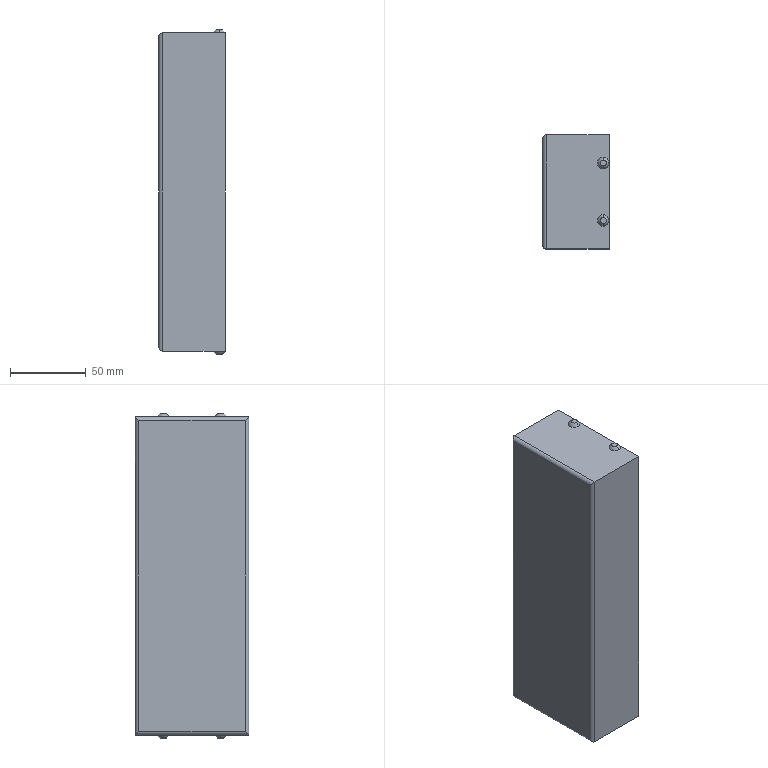Part | SolidWorks | features BaseBody 1 | 1 solid | 22 faces | box 44 x 75.3 x 214.7 mm | volume 696283 mm3 | plane 10 | torus 8 | cylinder 4 | commonest cylinder face diameters 5 x4
STEP:
#1=CARTESIAN_POINT('',(-0.2,19.5,-142.65));
#2=VERTEX_POINT('',#1);
#3=CARTESIAN_POINT('',(-7.8,19.5,-142.65));
#4=VERTEX_POINT('',#3);
#5=CARTESIAN_POINT('',(-4.,19.5,-142.65));
#6=DIRECTION('',(0.,0.,1.));
#7=DIRECTION('',(-1.,0.,0.));
#8=AXIS2_PLACEMENT_3D('',#5,#6,#7);
#9=CIRCLE('',#8,3.8);
#10=EDGE_CURVE('',#2,#4,#9,.T.);
#11=ORIENTED_EDGE('',*,*,#10,.F.);
#12=CARTESIAN_POINT('',(-2.,19.5,-144.85));
#13=VERTEX_POINT('',#12);
#14=CARTESIAN_POINT('',(-4.,19.5,-141.378));
#15=DIRECTION('',(0.,1.,0.));
#16=DIRECTION('',(-1.,0.,0.));
#17=AXIS2_PLACEMENT_3D('',#14,#15,#16);
#18=CIRCLE('',#17,4.007);
#19=EDGE_CURVE('',#2,#13,#18,.T.);
#20=ORIENTED_EDGE('',*,*,#19,.T.);
#21=CARTESIAN_POINT('',(-6.,19.5,-144.85));
#22=VERTEX_POINT('',#21);
#23=CARTESIAN_POINT('',(-4.,19.5,-144.85));
#24=DIRECTION('',(0.,0.,1.));
#25=DIRECTION('',(-1.,0.,0.));
#26=AXIS2_PLACEMENT_3D('',#23,#24,#25);
#27=CIRCLE('',#26,2.);
#28=EDGE_CURVE('',#13,#22,#27,.T.);
#29=ORIENTED_EDGE('',*,*,#28,.T.);
#30=CARTESIAN_POINT('',(-4.,19.5,-141.378));
#31=DIRECTION('',(0.,-1.,0.));
#32=DIRECTION('',(0.,0.,-1.));
#33=AXIS2_PLACEMENT_3D('',#30,#31,#32);
#34=CIRCLE('',#33,4.007);
#35=EDGE_CURVE('',#4,#22,#34,.T.);
#36=ORIENTED_EDGE('',*,*,#35,.F.);
#37=EDGE_LOOP('',(#11,#20,#29,#36));
#38=FACE_OUTER_BOUND('',#37,.T.);
#39=CARTESIAN_POINT('',(-4.,19.5,-141.378));
#40=DIRECTION('',(0.,0.,-1.));
#41=DIRECTION('',(-1.,0.,0.));
#42=AXIS2_PLACEMENT_3D('',#39,#40,#41);
#43=TOROIDAL_SURFACE('',#42,0.000391,4.007);
#44=ADVANCED_FACE('',(#38),#43,.T.);
#45=CARTESIAN_POINT('',(-0.2,57.5,-142.65));
#46=VERTEX_POINT('',#45);
#47=CARTESIAN_POINT('',(-7.8,57.5,-142.65));
#48=VERTEX_POINT('',#47);
#49=CARTESIAN_POINT('',(-4.,57.5,-142.65));
#50=DIRECTION('',(0.,0.,1.));
#51=DIRECTION('',(-1.,0.,0.));
#52=AXIS2_PLACEMENT_3D('',#49,#50,#51);
#53=CIRCLE('',#52,3.8);
#54=EDGE_CURVE('',#46,#48,#53,.T.);
#55=ORIENTED_EDGE('',*,*,#54,.F.);
#56=CARTESIAN_POINT('',(-2.,57.5,-144.85));
#57=VERTEX_POINT('',#56);
#58=CARTESIAN_POINT('',(-4.,57.5,-141.378));
#59=DIRECTION('',(0.,1.,0.));
#60=DIRECTION('',(-1.,0.,0.));
#61=AXIS2_PLACEMENT_3D('',#58,#59,#60);
#62=CIRCLE('',#61,4.007);
#63=EDGE_CURVE('',#46,#57,#62,.T.);
#64=ORIENTED_EDGE('',*,*,#63,.T.);
#65=CARTESIAN_POINT('',(-6.,57.5,-144.85));
#66=VERTEX_POINT('',#65);
#67=CARTESIAN_POINT('',(-4.,57.5,-144.85));
#68=DIRECTION('',(0.,0.,1.));
#69=DIRECTION('',(-1.,0.,0.));
#70=AXIS2_PLACEMENT_3D('',#67,#68,#69);
#71=CIRCLE('',#70,2.);
#72=EDGE_CURVE('',#57,#66,#71,.T.);
#73=ORIENTED_EDGE('',*,*,#72,.T.);
#74=CARTESIAN_POINT('',(-4.,57.5,-141.378));
#75=DIRECTION('',(0.,-1.,0.));
#76=DIRECTION('',(0.,0.,-1.));
#77=AXIS2_PLACEMENT_3D('',#74,#75,#76);
#78=CIRCLE('',#77,4.007);
#79=EDGE_CURVE('',#48,#66,#78,.T.);
#80=ORIENTED_EDGE('',*,*,#79,.F.);
#81=EDGE_LOOP('',(#55,#64,#73,#80));
#82=FACE_OUTER_BOUND('',#81,.T.);
#83=CARTESIAN_POINT('',(-4.,57.5,-141.378));
#84=DIRECTION('',(0.,0.,-1.));
#85=DIRECTION('',(-1.,0.,0.));
#86=AXIS2_PLACEMENT_3D('',#83,#84,#85);
#87=TOROIDAL_SURFACE('',#86,0.000391,4.007);
#88=ADVANCED_FACE('',(#82),#87,.T.);
#89=CARTESIAN_POINT('',(-4.,59.5,69.85));
#90=VERTEX_POINT('',#89);
#91=CARTESIAN_POINT('',(-4.,55.5,69.85));
#92=VERTEX_POINT('',#91);
#93=CARTESIAN_POINT('',(-4.,57.5,69.85));
#94=DIRECTION('',(0.,0.,-1.));
#95=DIRECTION('',(0.,1.,0.));
#96=AXIS2_PLACEMENT_3D('',#93,#94,#95);
#97=CIRCLE('',#96,2.);
#98=EDGE_CURVE('',#90,#92,#97,.T.);
#99=ORIENTED_EDGE('',*,*,#98,.T.);
#100=CARTESIAN_POINT('',(-4.,53.7,67.65));
#101=VERTEX_POINT('',#100);
#102=CARTESIAN_POINT('',(-4.,57.5,66.378));
#103=DIRECTION('',(1.,0.,0.));
#104=DIRECTION('',(0.,1.,0.));
#105=AXIS2_PLACEMENT_3D('',#102,#103,#104);
#106=CIRCLE('',#105,4.007);
#107=EDGE_CURVE('',#92,#101,#106,.T.);
#108=ORIENTED_EDGE('',*,*,#107,.T.);
#109=CARTESIAN_POINT('',(-4.,61.3,67.65));
#110=VERTEX_POINT('',#109);
#111=CARTESIAN_POINT('',(-4.,57.5,67.65));
#112=DIRECTION('',(0.,0.,-1.));
#113=DIRECTION('',(0.,1.,0.));
#114=AXIS2_PLACEMENT_3D('',#111,#112,#113);
#115=CIRCLE('',#114,3.8);
#116=EDGE_CURVE('',#110,#101,#115,.T.);
#117=ORIENTED_EDGE('',*,*,#116,.F.);
#118=CARTESIAN_POINT('',(-4.,57.5,66.378));
#119=DIRECTION('',(-1.,0.,0.));
#120=DIRECTION('',(0.,0.,1.));
#121=AXIS2_PLACEMENT_3D('',#118,#119,#120);
#122=CIRCLE('',#121,4.007);
#123=EDGE_CURVE('',#90,#110,#122,.T.);
#124=ORIENTED_EDGE('',*,*,#123,.F.);
#125=EDGE_LOOP('',(#99,#108,#117,#124));
#126=FACE_OUTER_BOUND('',#125,.T.);
#127=CARTESIAN_POINT('',(-4.,57.5,66.378));
#128=DIRECTION('',(0.,0.,-1.));
#129=DIRECTION('',(0.,1.,0.));
#130=AXIS2_PLACEMENT_3D('',#127,#128,#129);
#131=TOROIDAL_SURFACE('',#130,0.000391,4.007);
#132=ADVANCED_FACE('',(#126),#131,.T.);
#133=CARTESIAN_POINT('',(-4.,21.5,69.85));
#134=VERTEX_POINT('',#133);
#135=CARTESIAN_POINT('',(-4.,17.5,69.85));
#136=VERTEX_POINT('',#135);
#137=CARTESIAN_POINT('',(-4.,19.5,69.85));
#138=DIRECTION('',(0.,0.,-1.));
#139=DIRECTION('',(0.,1.,0.));
#140=AXIS2_PLACEMENT_3D('',#137,#138,#139);
#141=CIRCLE('',#140,2.);
#142=EDGE_CURVE('',#134,#136,#141,.T.);
#143=ORIENTED_EDGE('',*,*,#142,.T.);
#144=CARTESIAN_POINT('',(-4.,15.7,67.65));
#145=VERTEX_POINT('',#144);
#146=CARTESIAN_POINT('',(-4.,19.5,66.378));
#147=DIRECTION('',(1.,0.,0.));
#148=DIRECTION('',(0.,1.,0.));
#149=AXIS2_PLACEMENT_3D('',#146,#147,#148);
#150=CIRCLE('',#149,4.007);
#151=EDGE_CURVE('',#136,#145,#150,.T.);
#152=ORIENTED_EDGE('',*,*,#151,.T.);
#153=CARTESIAN_POINT('',(-4.,23.3,67.65));
#154=VERTEX_POINT('',#153);
#155=CARTESIAN_POINT('',(-4.,19.5,67.65));
#156=DIRECTION('',(0.,0.,-1.));
#157=DIRECTION('',(0.,1.,0.));
#158=AXIS2_PLACEMENT_3D('',#155,#156,#157);
#159=CIRCLE('',#158,3.8);
#160=EDGE_CURVE('',#154,#145,#159,.T.);
#161=ORIENTED_EDGE('',*,*,#160,.F.);
#162=CARTESIAN_POINT('',(-4.,19.5,66.378));
#163=DIRECTION('',(-1.,0.,0.));
#164=DIRECTION('',(0.,0.,1.));
#165=AXIS2_PLACEMENT_3D('',#162,#163,#164);
#166=CIRCLE('',#165,4.007);
#167=EDGE_CURVE('',#134,#154,#166,.T.);
#168=ORIENTED_EDGE('',*,*,#167,.F.);
#169=EDGE_LOOP('',(#143,#152,#161,#168));
#170=FACE_OUTER_BOUND('',#169,.T.);
#171=CARTESIAN_POINT('',(-4.,19.5,66.378));
#172=DIRECTION('',(0.,0.,-1.));
#173=DIRECTION('',(0.,1.,0.));
#174=AXIS2_PLACEMENT_3D('',#171,#172,#173);
#175=TOROIDAL_SURFACE('',#174,0.000391,4.007);
#176=ADVANCED_FACE('',(#170),#175,.T.);
#177=CARTESIAN_POINT('',(0.,0.85,-142.65));
#178=VERTEX_POINT('',#177);
#179=CARTESIAN_POINT('',(0.,76.15,-142.65));
#180=VERTEX_POINT('',#179);
#181=CARTESIAN_POINT('',(0.,0.,-142.65));
#182=DIRECTION('',(0.,1.,0.));
#183=VECTOR('',#182,1000.);
#184=LINE('',#181,#183);
#185=EDGE_CURVE('',#178,#180,#184,.T.);
#186=ORIENTED_EDGE('',*,*,#185,.T.);
#187=CARTESIAN_POINT('',(0.,76.15,67.65));
#188=VERTEX_POINT('',#187);
#189=CARTESIAN_POINT('',(0.,76.15,0.));
#190=DIRECTION('',(0.,0.,1.));
#191=VECTOR('',#190,1000.);
#192=LINE('',#189,#191);
#193=EDGE_CURVE('',#180,#188,#192,.T.);
#194=ORIENTED_EDGE('',*,*,#193,.T.);
#195=CARTESIAN_POINT('',(0.,0.85,67.65));
#196=VERTEX_POINT('',#195);
#197=CARTESIAN_POINT('',(0.,0.,67.65));
#198=DIRECTION('',(0.,-1.,0.));
#199=VECTOR('',#198,1000.);
#200=LINE('',#197,#199);
#201=EDGE_CURVE('',#188,#196,#200,.T.);
#202=ORIENTED_EDGE('',*,*,#201,.T.);
#203=CARTESIAN_POINT('',(0.,0.85,0.));
#204=DIRECTION('',(0.,0.,-1.));
#205=VECTOR('',#204,1000.);
#206=LINE('',#203,#205);
#207=EDGE_CURVE('',#196,#178,#206,.T.);
#208=ORIENTED_EDGE('',*,*,#207,.T.);
#209=EDGE_LOOP('',(#186,#194,#202,#208));
#210=FACE_OUTER_BOUND('',#209,.T.);
#211=CARTESIAN_POINT('',(0.,0.,0.));
#212=DIRECTION('',(1.,0.,0.));
#213=DIRECTION('',(0.,0.,-1.));
#214=AXIS2_PLACEMENT_3D('',#211,#212,#213);
#215=PLANE('',#214);
#216=ADVANCED_FACE('',(#210),#215,.T.);
#217=CARTESIAN_POINT('',(-41.5,76.15,67.65));
#218=VERTEX_POINT('',#217);
#219=CARTESIAN_POINT('',(-44.,76.15,67.65));
#220=DIRECTION('',(1.,0.,0.));
#221=VECTOR('',#220,1000.);
#222=LINE('',#219,#221);
#223=EDGE_CURVE('',#218,#188,#222,.T.);
#224=ORIENTED_EDGE('',*,*,#223,.T.);
#225=ORIENTED_EDGE('',*,*,#193,.F.);
#226=CARTESIAN_POINT('',(-41.5,76.15,-142.65));
#227=VERTEX_POINT('',#226);
#228=CARTESIAN_POINT('',(-44.,76.15,-142.65));
#229=DIRECTION('',(-1.,0.,0.));
#230=VECTOR('',#229,1000.);
#231=LINE('',#228,#230);
#232=EDGE_CURVE('',#180,#227,#231,.T.);
#233=ORIENTED_EDGE('',*,*,#232,.T.);
#234=CARTESIAN_POINT('',(-41.5,76.15,-142.65));
#235=DIRECTION('',(0.,0.,1.));
#236=VECTOR('',#235,1000.);
#237=LINE('',#234,#236);
#238=EDGE_CURVE('',#227,#218,#237,.T.);
#239=ORIENTED_EDGE('',*,*,#238,.T.);
#240=EDGE_LOOP('',(#224,#225,#233,#239));
#241=FACE_OUTER_BOUND('',#240,.T.);
#242=CARTESIAN_POINT('',(-44.,76.15,-142.65));
#243=DIRECTION('',(0.,1.,0.));
#244=DIRECTION('',(0.,0.,1.));
#245=AXIS2_PLACEMENT_3D('',#242,#243,#244);
#246=PLANE('',#245);
#247=ADVANCED_FACE('',(#241),#246,.T.);
#248=ORIENTED_EDGE('',*,*,#232,.F.);
#249=ORIENTED_EDGE('',*,*,#185,.F.);
#250=CARTESIAN_POINT('',(-41.5,0.85,-142.65));
#251=VERTEX_POINT('',#250);
#252=CARTESIAN_POINT('',(-44.,0.85,-142.65));
#253=DIRECTION('',(-1.,0.,0.));
#254=VECTOR('',#253,1000.);
#255=LINE('',#252,#254);
#256=EDGE_CURVE('',#178,#251,#255,.T.);
#257=ORIENTED_EDGE('',*,*,#256,.T.);
#258=CARTESIAN_POINT('',(-41.5,0.85,-142.65));
#259=DIRECTION('',(0.,1.,0.));
#260=VECTOR('',#259,1000.);
#261=LINE('',#258,#260);
#262=EDGE_CURVE('',#251,#227,#261,.T.);
#263=ORIENTED_EDGE('',*,*,#262,.T.);
#264=EDGE_LOOP('',(#248,#249,#257,#263));
#265=FACE_OUTER_BOUND('',#264,.T.);
#266=CARTESIAN_POINT('',(-4.,19.5,-142.65));
#267=DIRECTION('',(0.,0.,1.));
#268=DIRECTION('',(-1.,0.,0.));
#269=AXIS2_PLACEMENT_3D('',#266,#267,#268);
#270=CIRCLE('',#269,3.8);
#271=EDGE_CURVE('',#4,#2,#270,.T.);
#272=ORIENTED_EDGE('',*,*,#271,.T.);
#273=ORIENTED_EDGE('',*,*,#10,.T.);
#274=EDGE_LOOP('',(#272,#273));
#275=FACE_BOUND('',#274,.T.);
#276=CARTESIAN_POINT('',(-4.,57.5,-142.65));
#277=DIRECTION('',(0.,0.,1.));
#278=DIRECTION('',(-1.,0.,0.));
#279=AXIS2_PLACEMENT_3D('',#276,#277,#278);
#280=CIRCLE('',#279,3.8);
#281=EDGE_CURVE('',#48,#46,#280,.T.);
#282=ORIENTED_EDGE('',*,*,#281,.T.);
#283=ORIENTED_EDGE('',*,*,#54,.T.);
#284=EDGE_LOOP('',(#282,#283));
#285=FACE_BOUND('',#284,.T.);
#286=CARTESIAN_POINT('',(-44.,0.85,-142.65));
#287=DIRECTION('',(0.,0.,-1.));
#288=DIRECTION('',(-1.,0.,0.));
#289=AXIS2_PLACEMENT_3D('',#286,#287,#288);
#290=PLANE('',#289);
#291=ADVANCED_FACE('',(#265,#275,#285),#290,.T.);
#292=ORIENTED_EDGE('',*,*,#256,.F.);
#293=ORIENTED_EDGE('',*,*,#207,.F.);
#294=CARTESIAN_POINT('',(-41.5,0.85,67.65));
#295=VERTEX_POINT('',#294);
#296=CARTESIAN_POINT('',(-44.,0.85,67.65));
#297=DIRECTION('',(-1.,0.,0.));
#298=VECTOR('',#297,1000.);
#299=LINE('',#296,#298);
#300=EDGE_CURVE('',#196,#295,#299,.T.);
#301=ORIENTED_EDGE('',*,*,#300,.T.);
#302=CARTESIAN_POINT('',(-41.5,0.85,67.65));
#303=DIRECTION('',(0.,0.,-1.));
#304=VECTOR('',#303,1000.);
#305=LINE('',#302,#304);
#306=EDGE_CURVE('',#295,#251,#305,.T.);
#307=ORIENTED_EDGE('',*,*,#306,.T.);
#308=EDGE_LOOP('',(#292,#293,#301,#307));
#309=FACE_OUTER_BOUND('',#308,.T.);
#310=CARTESIAN_POINT('',(-44.,0.85,67.65));
#311=DIRECTION('',(0.,-1.,0.));
#312=DIRECTION('',(0.,0.,-1.));
#313=AXIS2_PLACEMENT_3D('',#310,#311,#312);
#314=PLANE('',#313);
#315=ADVANCED_FACE('',(#309),#314,.T.);
#316=ORIENTED_EDGE('',*,*,#300,.F.);
#317=ORIENTED_EDGE('',*,*,#201,.F.);
#318=ORIENTED_EDGE('',*,*,#223,.F.);
#319=CARTESIAN_POINT('',(-41.5,76.15,67.65));
#320=DIRECTION('',(0.,-1.,0.));
#321=VECTOR('',#320,1000.);
#322=LINE('',#319,#321);
#323=EDGE_CURVE('',#218,#295,#322,.T.);
#324=ORIENTED_EDGE('',*,*,#323,.T.);
#325=EDGE_LOOP('',(#316,#317,#318,#324));
#326=FACE_OUTER_BOUND('',#325,.T.);
#327=ORIENTED_EDGE('',*,*,#116,.T.);
#328=CARTESIAN_POINT('',(-4.,57.5,67.65));
#329=DIRECTION('',(0.,0.,-1.));
#330=DIRECTION('',(0.,1.,0.));
#331=AXIS2_PLACEMENT_3D('',#328,#329,#330);
#332=CIRCLE('',#331,3.8);
#333=EDGE_CURVE('',#101,#110,#332,.T.);
#334=ORIENTED_EDGE('',*,*,#333,.T.);
#335=EDGE_LOOP('',(#327,#334));
#336=FACE_BOUND('',#335,.T.);
#337=ORIENTED_EDGE('',*,*,#160,.T.);
#338=CARTESIAN_POINT('',(-4.,19.5,67.65));
#339=DIRECTION('',(0.,0.,-1.));
#340=DIRECTION('',(0.,1.,0.));
#341=AXIS2_PLACEMENT_3D('',#338,#339,#340);
#342=CIRCLE('',#341,3.8);
#343=EDGE_CURVE('',#145,#154,#342,.T.);
#344=ORIENTED_EDGE('',*,*,#343,.T.);
#345=EDGE_LOOP('',(#337,#344));
#346=FACE_BOUND('',#345,.T.);
#347=CARTESIAN_POINT('',(-44.,76.15,67.65));
#348=DIRECTION('',(0.,0.,1.));
#349=DIRECTION('',(0.,-1.,0.));
#350=AXIS2_PLACEMENT_3D('',#347,#348,#349);
#351=PLANE('',#350);
#352=ADVANCED_FACE('',(#326,#336,#346),#351,.T.);
#353=CARTESIAN_POINT('',(-44.,73.65,65.15));
#354=VERTEX_POINT('',#353);
#355=CARTESIAN_POINT('',(-44.,73.65,65.15));
#356=CARTESIAN_POINT('',(-44.,75.114,66.614));
#357=CARTESIAN_POINT('',(-42.964,76.15,67.65));
#358=CARTESIAN_POINT('',(-41.5,76.15,67.65));
#359=(BOUNDED_CURVE()B_SPLINE_CURVE(3,(#355,#356,#357,#358),.UNSPECIFIED.,.F.,.F.)B_SPLINE_CURVE_WITH_KNOTS((4,4),(4.712,6.283),.UNSPECIFIED.)CURVE()GEOMETRIC_REPRESENTATION_ITEM()RATIONAL_B_SPLINE_CURVE((1.,0.8047,0.8047,1.))REPRESENTATION_ITEM(''));
#360=EDGE_CURVE('',#354,#218,#359,.T.);
#361=ORIENTED_EDGE('',*,*,#360,.T.);
#362=ORIENTED_EDGE('',*,*,#238,.F.);
#363=CARTESIAN_POINT('',(-44.,73.65,-140.15));
#364=VERTEX_POINT('',#363);
#365=CARTESIAN_POINT('',(-41.5,76.15,-142.65));
#366=CARTESIAN_POINT('',(-42.964,76.15,-142.65));
#367=CARTESIAN_POINT('',(-44.,75.114,-141.614));
#368=CARTESIAN_POINT('',(-44.,73.65,-140.15));
#369=(BOUNDED_CURVE()B_SPLINE_CURVE(3,(#365,#366,#367,#368),.UNSPECIFIED.,.F.,.F.)B_SPLINE_CURVE_WITH_KNOTS((4,4),(3.142,4.712),.UNSPECIFIED.)CURVE()GEOMETRIC_REPRESENTATION_ITEM()RATIONAL_B_SPLINE_CURVE((1.,0.8047,0.8047,1.))REPRESENTATION_ITEM(''));
#370=EDGE_CURVE('',#227,#364,#369,.T.);
#371=ORIENTED_EDGE('',*,*,#370,.T.);
#372=CARTESIAN_POINT('',(-44.,73.65,-142.65));
#373=DIRECTION('',(0.,0.,1.));
#374=VECTOR('',#373,1000.);
#375=LINE('',#372,#374);
#376=EDGE_CURVE('',#364,#354,#375,.T.);
#377=ORIENTED_EDGE('',*,*,#376,.T.);
#378=EDGE_LOOP('',(#361,#362,#371,#377));
#379=FACE_OUTER_BOUND('',#378,.T.);
#380=CARTESIAN_POINT('',(-41.5,73.65,-142.65));
#381=DIRECTION('',(0.,0.,1.));
#382=DIRECTION('',(1.,0.,0.));
#383=AXIS2_PLACEMENT_3D('',#380,#381,#382);
#384=CYLINDRICAL_SURFACE('',#383,2.5);
#385=ADVANCED_FACE('',(#379),#384,.T.);
#386=CARTESIAN_POINT('',(-44.,3.35,-140.15));
#387=VERTEX_POINT('',#386);
#388=CARTESIAN_POINT('',(-41.5,0.85,-142.65));
#389=CARTESIAN_POINT('',(-42.964,0.85,-142.65));
#390=CARTESIAN_POINT('',(-44.,1.886,-141.614));
#391=CARTESIAN_POINT('',(-44.,3.35,-140.15));
#392=(BOUNDED_CURVE()B_SPLINE_CURVE(3,(#388,#389,#390,#391),.UNSPECIFIED.,.F.,.F.)B_SPLINE_CURVE_WITH_KNOTS((4,4),(3.142,4.712),.UNSPECIFIED.)CURVE()GEOMETRIC_REPRESENTATION_ITEM()RATIONAL_B_SPLINE_CURVE((1.,0.8047,0.8047,1.))REPRESENTATION_ITEM(''));
#393=EDGE_CURVE('',#251,#387,#392,.T.);
#394=ORIENTED_EDGE('',*,*,#393,.T.);
#395=CARTESIAN_POINT('',(-44.,0.85,-140.15));
#396=DIRECTION('',(0.,1.,0.));
#397=VECTOR('',#396,1000.);
#398=LINE('',#395,#397);
#399=EDGE_CURVE('',#387,#364,#398,.T.);
#400=ORIENTED_EDGE('',*,*,#399,.T.);
#401=ORIENTED_EDGE('',*,*,#370,.F.);
#402=ORIENTED_EDGE('',*,*,#262,.F.);
#403=EDGE_LOOP('',(#394,#400,#401,#402));
#404=FACE_OUTER_BOUND('',#403,.T.);
#405=CARTESIAN_POINT('',(-41.5,0.85,-140.15));
#406=DIRECTION('',(0.,1.,0.));
#407=DIRECTION('',(0.,0.,1.));
#408=AXIS2_PLACEMENT_3D('',#405,#406,#407);
#409=CYLINDRICAL_SURFACE('',#408,2.5);
#410=ADVANCED_FACE('',(#404),#409,.T.);
#411=ORIENTED_EDGE('',*,*,#19,.F.);
#412=ORIENTED_EDGE('',*,*,#271,.F.);
#413=ORIENTED_EDGE('',*,*,#35,.T.);
#414=CARTESIAN_POINT('',(-4.,19.5,-144.85));
#415=DIRECTION('',(0.,0.,1.));
#416=DIRECTION('',(-1.,0.,0.));
#417=AXIS2_PLACEMENT_3D('',#414,#415,#416);
#418=CIRCLE('',#417,2.);
#419=EDGE_CURVE('',#22,#13,#418,.T.);
#420=ORIENTED_EDGE('',*,*,#419,.T.);
#421=EDGE_LOOP('',(#411,#412,#413,#420));
#422=FACE_OUTER_BOUND('',#421,.T.);
#423=CARTESIAN_POINT('',(-4.,19.5,-141.378));
#424=DIRECTION('',(0.,0.,-1.));
#425=DIRECTION('',(-1.,0.,0.));
#426=AXIS2_PLACEMENT_3D('',#423,#424,#425);
#427=TOROIDAL_SURFACE('',#426,0.000391,4.007);
#428=ADVANCED_FACE('',(#422),#427,.T.);
#429=ORIENTED_EDGE('',*,*,#63,.F.);
#430=ORIENTED_EDGE('',*,*,#281,.F.);
#431=ORIENTED_EDGE('',*,*,#79,.T.);
#432=CARTESIAN_POINT('',(-4.,57.5,-144.85));
#433=DIRECTION('',(0.,0.,1.));
#434=DIRECTION('',(-1.,0.,0.));
#435=AXIS2_PLACEMENT_3D('',#432,#433,#434);
#436=CIRCLE('',#435,2.);
#437=EDGE_CURVE('',#66,#57,#436,.T.);
#438=ORIENTED_EDGE('',*,*,#437,.T.);
#439=EDGE_LOOP('',(#429,#430,#431,#438));
#440=FACE_OUTER_BOUND('',#439,.T.);
#441=CARTESIAN_POINT('',(-4.,57.5,-141.378));
#442=DIRECTION('',(0.,0.,-1.));
#443=DIRECTION('',(-1.,0.,0.));
#444=AXIS2_PLACEMENT_3D('',#441,#442,#443);
#445=TOROIDAL_SURFACE('',#444,0.000391,4.007);
#446=ADVANCED_FACE('',(#440),#445,.T.);
#447=ORIENTED_EDGE('',*,*,#393,.F.);
#448=ORIENTED_EDGE('',*,*,#306,.F.);
#449=CARTESIAN_POINT('',(-44.,3.35,65.15));
#450=VERTEX_POINT('',#449);
#451=CARTESIAN_POINT('',(-41.5,0.85,67.65));
#452=CARTESIAN_POINT('',(-42.964,0.85,67.65));
#453=CARTESIAN_POINT('',(-44.,1.886,66.614));
#454=CARTESIAN_POINT('',(-44.,3.35,65.15));
#455=(BOUNDED_CURVE()B_SPLINE_CURVE(3,(#451,#452,#453,#454),.UNSPECIFIED.,.F.,.F.)B_SPLINE_CURVE_WITH_KNOTS((4,4),(3.142,4.712),.UNSPECIFIED.)CURVE()GEOMETRIC_REPRESENTATION_ITEM()RATIONAL_B_SPLINE_CURVE((1.,0.8047,0.8047,1.))REPRESENTATION_ITEM(''));
#456=EDGE_CURVE('',#295,#450,#455,.T.);
#457=ORIENTED_EDGE('',*,*,#456,.T.);
#458=CARTESIAN_POINT('',(-44.,3.35,67.65));
#459=DIRECTION('',(0.,0.,-1.));
#460=VECTOR('',#459,1000.);
#461=LINE('',#458,#460);
#462=EDGE_CURVE('',#450,#387,#461,.T.);
#463=ORIENTED_EDGE('',*,*,#462,.T.);
#464=EDGE_LOOP('',(#447,#448,#457,#463));
#465=FACE_OUTER_BOUND('',#464,.T.);
#466=CARTESIAN_POINT('',(-41.5,3.35,67.65));
#467=DIRECTION('',(0.,0.,-1.));
#468=DIRECTION('',(0.,1.,0.));
#469=AXIS2_PLACEMENT_3D('',#466,#467,#468);
#470=CYLINDRICAL_SURFACE('',#469,2.5);
#471=ADVANCED_FACE('',(#465),#470,.T.);
#472=ORIENTED_EDGE('',*,*,#456,.F.);
#473=ORIENTED_EDGE('',*,*,#323,.F.);
#474=ORIENTED_EDGE('',*,*,#360,.F.);
#475=CARTESIAN_POINT('',(-44.,76.15,65.15));
#476=DIRECTION('',(0.,-1.,0.));
#477=VECTOR('',#476,1000.);
#478=LINE('',#475,#477);
#479=EDGE_CURVE('',#354,#450,#478,.T.);
#480=ORIENTED_EDGE('',*,*,#479,.T.);
#481=EDGE_LOOP('',(#472,#473,#474,#480));
#482=FACE_OUTER_BOUND('',#481,.T.);
#483=CARTESIAN_POINT('',(-41.5,76.15,65.15));
#484=DIRECTION('',(0.,-1.,0.));
#485=DIRECTION('',(0.,0.,-1.));
#486=AXIS2_PLACEMENT_3D('',#483,#484,#485);
#487=CYLINDRICAL_SURFACE('',#486,2.5);
#488=ADVANCED_FACE('',(#482),#487,.T.);
#489=ORIENTED_EDGE('',*,*,#107,.F.);
#490=CARTESIAN_POINT('',(-4.,57.5,69.85));
#491=DIRECTION('',(0.,0.,-1.));
#492=DIRECTION('',(0.,1.,0.));
#493=AXIS2_PLACEMENT_3D('',#490,#491,#492);
#494=CIRCLE('',#493,2.);
#495=EDGE_CURVE('',#92,#90,#494,.T.);
#496=ORIENTED_EDGE('',*,*,#495,.T.);
#497=ORIENTED_EDGE('',*,*,#123,.T.);
#498=ORIENTED_EDGE('',*,*,#333,.F.);
#499=EDGE_LOOP('',(#489,#496,#497,#498));
#500=FACE_OUTER_BOUND('',#499,.T.);
#501=CARTESIAN_POINT('',(-4.,57.5,66.378));
#502=DIRECTION('',(0.,0.,-1.));
#503=DIRECTION('',(0.,1.,0.));
#504=AXIS2_PLACEMENT_3D('',#501,#502,#503);
#505=TOROIDAL_SURFACE('',#504,0.000391,4.007);
#506=ADVANCED_FACE('',(#500),#505,.T.);
#507=ORIENTED_EDGE('',*,*,#151,.F.);
#508=CARTESIAN_POINT('',(-4.,19.5,69.85));
#509=DIRECTION('',(0.,0.,-1.));
#510=DIRECTION('',(0.,1.,0.));
#511=AXIS2_PLACEMENT_3D('',#508,#509,#510);
#512=CIRCLE('',#511,2.);
#513=EDGE_CURVE('',#136,#134,#512,.T.);
#514=ORIENTED_EDGE('',*,*,#513,.T.);
#515=ORIENTED_EDGE('',*,*,#167,.T.);
#516=ORIENTED_EDGE('',*,*,#343,.F.);
#517=EDGE_LOOP('',(#507,#514,#515,#516));
#518=FACE_OUTER_BOUND('',#517,.T.);
#519=CARTESIAN_POINT('',(-4.,19.5,66.378));
#520=DIRECTION('',(0.,0.,-1.));
#521=DIRECTION('',(0.,1.,0.));
#522=AXIS2_PLACEMENT_3D('',#519,#520,#521);
#523=TOROIDAL_SURFACE('',#522,0.000391,4.007);
#524=ADVANCED_FACE('',(#518),#523,.T.);
#525=ORIENTED_EDGE('',*,*,#462,.F.);
#526=ORIENTED_EDGE('',*,*,#479,.F.);
#527=ORIENTED_EDGE('',*,*,#376,.F.);
#528=ORIENTED_EDGE('',*,*,#399,.F.);
#529=EDGE_LOOP('',(#525,#526,#527,#528));
#530=FACE_OUTER_BOUND('',#529,.T.);
#531=CARTESIAN_POINT('',(-44.,0.,0.));
#532=DIRECTION('',(1.,0.,0.));
#533=DIRECTION('',(0.,0.,-1.));
#534=AXIS2_PLACEMENT_3D('',#531,#532,#533);
#535=PLANE('',#534);
#536=ADVANCED_FACE('',(#530),#535,.F.);
#537=ORIENTED_EDGE('',*,*,#419,.F.);
#538=ORIENTED_EDGE('',*,*,#28,.F.);
#539=EDGE_LOOP('',(#537,#538));
#540=FACE_OUTER_BOUND('',#539,.T.);
#541=CARTESIAN_POINT('',(-4.,21.5,-144.85));
#542=DIRECTION('',(0.,0.,1.));
#543=DIRECTION('',(1.,0.,0.));
#544=AXIS2_PLACEMENT_3D('',#541,#542,#543);
#545=PLANE('',#544);
#546=ADVANCED_FACE('',(#540),#545,.F.);
#547=ORIENTED_EDGE('',*,*,#437,.F.);
#548=ORIENTED_EDGE('',*,*,#72,.F.);
#549=EDGE_LOOP('',(#547,#548));
#550=FACE_OUTER_BOUND('',#549,.T.);
#551=CARTESIAN_POINT('',(-4.,59.5,-144.85));
#552=DIRECTION('',(0.,0.,1.));
#553=DIRECTION('',(1.,0.,0.));
#554=AXIS2_PLACEMENT_3D('',#551,#552,#553);
#555=PLANE('',#554);
#556=ADVANCED_FACE('',(#550),#555,.F.);
#557=ORIENTED_EDGE('',*,*,#98,.F.);
#558=ORIENTED_EDGE('',*,*,#495,.F.);
#559=EDGE_LOOP('',(#557,#558));
#560=FACE_OUTER_BOUND('',#559,.T.);
#561=CARTESIAN_POINT('',(-4.,57.5,69.85));
#562=DIRECTION('',(0.,0.,-1.));
#563=DIRECTION('',(-1.,0.,0.));
#564=AXIS2_PLACEMENT_3D('',#561,#562,#563);
#565=PLANE('',#564);
#566=ADVANCED_FACE('',(#560),#565,.F.);
#567=ORIENTED_EDGE('',*,*,#142,.F.);
#568=ORIENTED_EDGE('',*,*,#513,.F.);
#569=EDGE_LOOP('',(#567,#568));
#570=FACE_OUTER_BOUND('',#569,.T.);
#571=CARTESIAN_POINT('',(-4.,19.5,69.85));
#572=DIRECTION('',(0.,0.,-1.));
#573=DIRECTION('',(-1.,0.,0.));
#574=AXIS2_PLACEMENT_3D('',#571,#572,#573);
#575=PLANE('',#574);
#576=ADVANCED_FACE('',(#570),#575,.F.);
#577=CLOSED_SHELL('',(#44,#88,#132,#176,#216,#247,#291,#315,#352,#385,#410,#428,#446,#471,#488,#506,#524,#536,#546,#556,#566,#576));
#578=MANIFOLD_SOLID_BREP('',#577);
#579=CARTESIAN_POINT('',(0.,0.,0.));
#580=DIRECTION('',(0.,0.,1.));
#581=DIRECTION('',(1.,0.,0.));
#582=AXIS2_PLACEMENT_3D('',#579,#580,#581);
#583=(LENGTH_UNIT()NAMED_UNIT(*)SI_UNIT(.MILLI.,.METRE.));
#584=UNCERTAINTY_MEASURE_WITH_UNIT(LENGTH_MEASURE(0.00001),#583,'','');
#585=(NAMED_UNIT(*)PLANE_ANGLE_UNIT()SI_UNIT($,.RADIAN.));
#586=(NAMED_UNIT(*)SI_UNIT($,.STERADIAN.)SOLID_ANGLE_UNIT());
#587=(GEOMETRIC_REPRESENTATION_CONTEXT(3)GLOBAL_UNCERTAINTY_ASSIGNED_CONTEXT((#584))GLOBAL_UNIT_ASSIGNED_CONTEXT((#583,#585,#586))REPRESENTATION_CONTEXT('',''));
#588=ADVANCED_BREP_SHAPE_REPRESENTATION('',(#578,#582),#587);